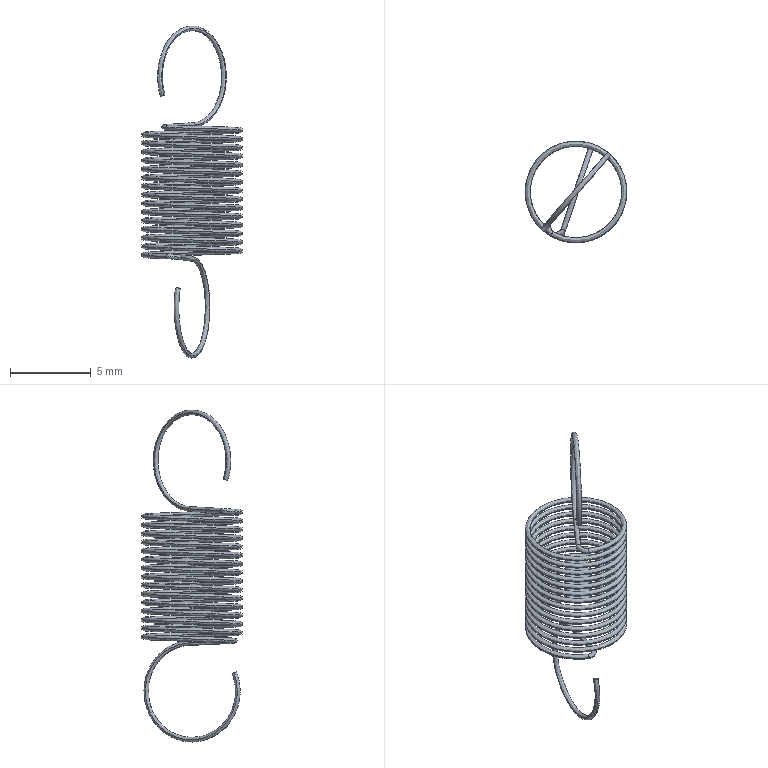Part | SolidWorks | features 3DProfileFeature 2, MacroFeature 1 | 1 solid | 16 faces | box 6.3 x 6.3 x 20.605 mm | volume 22.571 mm3 | spline 14 | plane 2